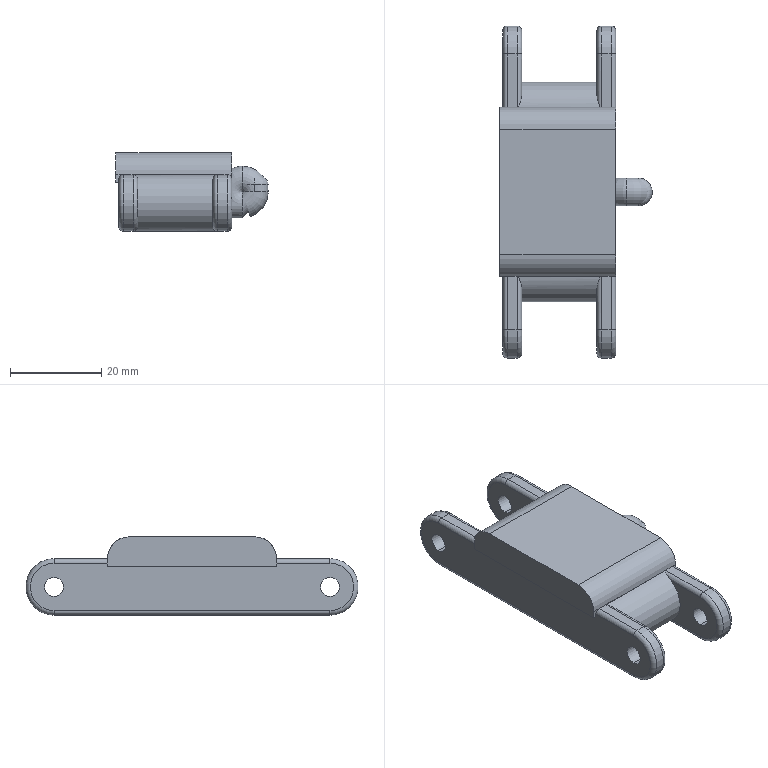Part | SolidWorks | features ICE 5, 3DProfileFeature 2, Fillet 2, Extrusion 1, LPattern 1, Scale 1, Sweep 1 | 1 solid | 114 faces | box 33.423 x 72.908 x 17.17 mm | volume 16126 mm3 | plane 66 | cylinder 36 | torus 12 | commonest cylinder face diameters 1.981 x14 4.127 x8 12.383 x5 6.09 x4 8.255 x2 9.576 x2